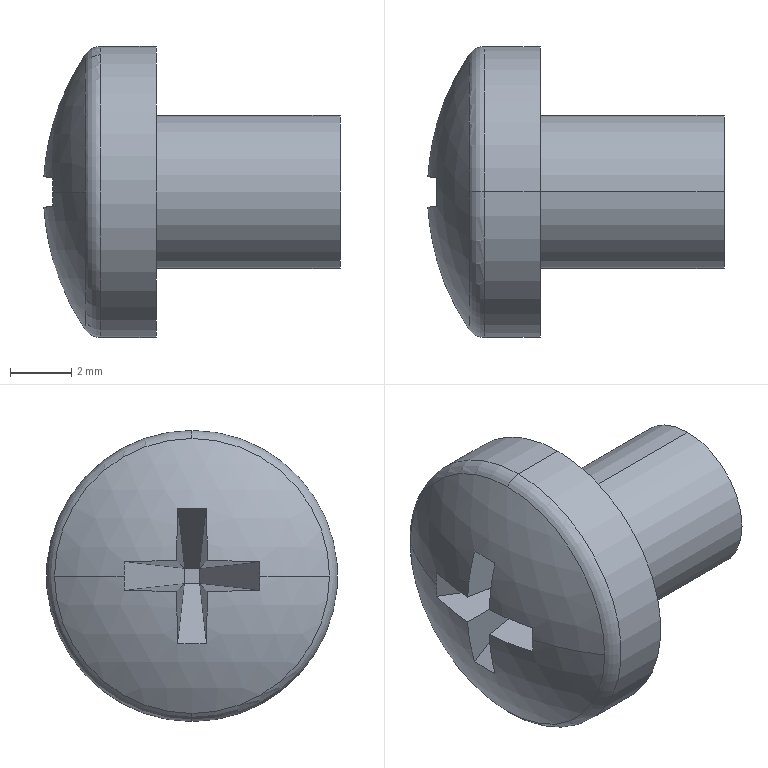Part | STEP file | pan cross head_am_B18.6.7M - M5 x 0.8 x 6 Type I Cross Recessed PHMS --6N | 1 solid | 23 faces | box 9.669 x 9.5 x 9.5 mm | volume 316.024 mm3 | plane 15 | cylinder 4 | torus 2 | sphere 2 | commonest cylinder face diameters 5 x2 9.5 x2